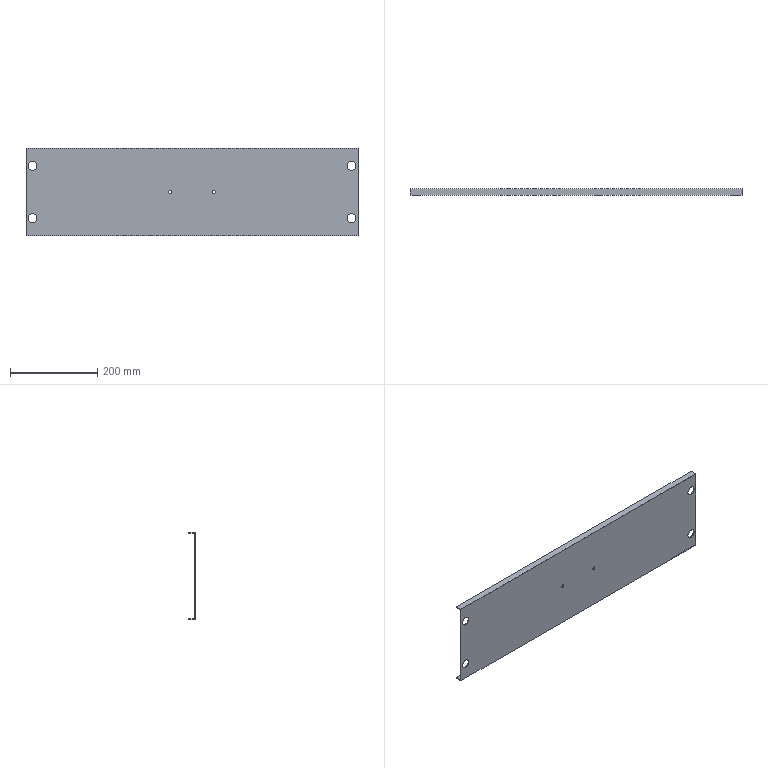Part | SolidWorks | features BaseBody 1 | 1 solid | 22 faces | box 760 x 15 x 200 mm | volume 340844 mm3 | cylinder 12 | plane 10 | commonest cylinder face diameters 20 x8 7.2 x4
STEP:
#1=CARTESIAN_POINT('',(181.946,-3036.473,1814.721));
#2=VERTEX_POINT('',#1);
#3=CARTESIAN_POINT('',(181.946,-3036.473,1794.721));
#4=VERTEX_POINT('',#3);
#5=CARTESIAN_POINT('',(181.946,-3036.473,1804.721));
#6=DIRECTION('',(0.,-1.,0.));
#7=DIRECTION('',(0.,0.,-1.));
#8=AXIS2_PLACEMENT_3D('',#5,#6,#7);
#9=CIRCLE('',#8,10.);
#10=EDGE_CURVE('',#2,#4,#9,.T.);
#11=ORIENTED_EDGE('',*,*,#10,.F.);
#12=CARTESIAN_POINT('',(181.946,-3038.473,1814.721));
#13=VERTEX_POINT('',#12);
#14=CARTESIAN_POINT('',(181.946,-3062.967,1814.721));
#15=DIRECTION('',(0.,-1.,0.));
#16=VECTOR('',#15,1000.);
#17=LINE('',#14,#16);
#18=EDGE_CURVE('',#2,#13,#17,.T.);
#19=ORIENTED_EDGE('',*,*,#18,.T.);
#20=CARTESIAN_POINT('',(181.946,-3038.473,1794.721));
#21=VERTEX_POINT('',#20);
#22=CARTESIAN_POINT('',(181.946,-3038.473,1804.721));
#23=DIRECTION('',(0.,1.,0.));
#24=DIRECTION('',(0.,0.,-1.));
#25=AXIS2_PLACEMENT_3D('',#22,#23,#24);
#26=CIRCLE('',#25,10.);
#27=EDGE_CURVE('',#21,#13,#26,.T.);
#28=ORIENTED_EDGE('',*,*,#27,.F.);
#29=CARTESIAN_POINT('',(181.946,-3062.967,1794.721));
#30=DIRECTION('',(0.,-1.,0.));
#31=VECTOR('',#30,1000.);
#32=LINE('',#29,#31);
#33=EDGE_CURVE('',#4,#21,#32,.T.);
#34=ORIENTED_EDGE('',*,*,#33,.F.);
#35=EDGE_LOOP('',(#11,#19,#28,#34));
#36=FACE_OUTER_BOUND('',#35,.T.);
#37=CARTESIAN_POINT('',(181.946,-3062.967,1804.721));
#38=DIRECTION('',(0.,-1.,0.));
#39=DIRECTION('',(0.,0.,-1.));
#40=AXIS2_PLACEMENT_3D('',#37,#38,#39);
#41=CYLINDRICAL_SURFACE('',#40,10.);
#42=ADVANCED_FACE('',(#36),#41,.F.);
#43=CARTESIAN_POINT('',(911.946,-3038.473,1794.721));
#44=VERTEX_POINT('',#43);
#45=CARTESIAN_POINT('',(911.946,-3038.473,1814.721));
#46=VERTEX_POINT('',#45);
#47=CARTESIAN_POINT('',(911.946,-3038.473,1804.721));
#48=DIRECTION('',(0.,1.,0.));
#49=DIRECTION('',(0.,0.,1.));
#50=AXIS2_PLACEMENT_3D('',#47,#48,#49);
#51=CIRCLE('',#50,10.);
#52=EDGE_CURVE('',#44,#46,#51,.T.);
#53=ORIENTED_EDGE('',*,*,#52,.F.);
#54=CARTESIAN_POINT('',(911.946,-3036.473,1794.721));
#55=VERTEX_POINT('',#54);
#56=CARTESIAN_POINT('',(911.946,-3062.967,1794.721));
#57=DIRECTION('',(0.,1.,0.));
#58=VECTOR('',#57,1000.);
#59=LINE('',#56,#58);
#60=EDGE_CURVE('',#44,#55,#59,.T.);
#61=ORIENTED_EDGE('',*,*,#60,.T.);
#62=CARTESIAN_POINT('',(911.946,-3036.473,1814.721));
#63=VERTEX_POINT('',#62);
#64=CARTESIAN_POINT('',(911.946,-3036.473,1804.721));
#65=DIRECTION('',(0.,-1.,0.));
#66=DIRECTION('',(0.,0.,1.));
#67=AXIS2_PLACEMENT_3D('',#64,#65,#66);
#68=CIRCLE('',#67,10.);
#69=EDGE_CURVE('',#63,#55,#68,.T.);
#70=ORIENTED_EDGE('',*,*,#69,.F.);
#71=CARTESIAN_POINT('',(911.946,-3062.967,1814.721));
#72=DIRECTION('',(0.,1.,0.));
#73=VECTOR('',#72,1000.);
#74=LINE('',#71,#73);
#75=EDGE_CURVE('',#46,#63,#74,.T.);
#76=ORIENTED_EDGE('',*,*,#75,.F.);
#77=EDGE_LOOP('',(#53,#61,#70,#76));
#78=FACE_OUTER_BOUND('',#77,.T.);
#79=CARTESIAN_POINT('',(911.946,-3062.967,1804.721));
#80=DIRECTION('',(0.,1.,0.));
#81=DIRECTION('',(0.,0.,1.));
#82=AXIS2_PLACEMENT_3D('',#79,#80,#81);
#83=CYLINDRICAL_SURFACE('',#82,10.);
#84=ADVANCED_FACE('',(#78),#83,.F.);
#85=CARTESIAN_POINT('',(911.946,-3038.473,1674.721));
#86=VERTEX_POINT('',#85);
#87=CARTESIAN_POINT('',(911.946,-3038.473,1694.721));
#88=VERTEX_POINT('',#87);
#89=CARTESIAN_POINT('',(911.946,-3038.473,1684.721));
#90=DIRECTION('',(0.,1.,0.));
#91=DIRECTION('',(0.,0.,1.));
#92=AXIS2_PLACEMENT_3D('',#89,#90,#91);
#93=CIRCLE('',#92,10.);
#94=EDGE_CURVE('',#86,#88,#93,.T.);
#95=ORIENTED_EDGE('',*,*,#94,.F.);
#96=CARTESIAN_POINT('',(911.946,-3036.473,1674.721));
#97=VERTEX_POINT('',#96);
#98=CARTESIAN_POINT('',(911.946,-3062.967,1674.721));
#99=DIRECTION('',(0.,1.,0.));
#100=VECTOR('',#99,1000.);
#101=LINE('',#98,#100);
#102=EDGE_CURVE('',#86,#97,#101,.T.);
#103=ORIENTED_EDGE('',*,*,#102,.T.);
#104=CARTESIAN_POINT('',(911.946,-3036.473,1694.721));
#105=VERTEX_POINT('',#104);
#106=CARTESIAN_POINT('',(911.946,-3036.473,1684.721));
#107=DIRECTION('',(0.,-1.,0.));
#108=DIRECTION('',(0.,0.,1.));
#109=AXIS2_PLACEMENT_3D('',#106,#107,#108);
#110=CIRCLE('',#109,10.);
#111=EDGE_CURVE('',#105,#97,#110,.T.);
#112=ORIENTED_EDGE('',*,*,#111,.F.);
#113=CARTESIAN_POINT('',(911.946,-3062.967,1694.721));
#114=DIRECTION('',(0.,1.,0.));
#115=VECTOR('',#114,1000.);
#116=LINE('',#113,#115);
#117=EDGE_CURVE('',#88,#105,#116,.T.);
#118=ORIENTED_EDGE('',*,*,#117,.F.);
#119=EDGE_LOOP('',(#95,#103,#112,#118));
#120=FACE_OUTER_BOUND('',#119,.T.);
#121=CARTESIAN_POINT('',(911.946,-3062.967,1684.721));
#122=DIRECTION('',(0.,1.,0.));
#123=DIRECTION('',(0.,0.,1.));
#124=AXIS2_PLACEMENT_3D('',#121,#122,#123);
#125=CYLINDRICAL_SURFACE('',#124,10.);
#126=ADVANCED_FACE('',(#120),#125,.F.);
#127=CARTESIAN_POINT('',(181.946,-3036.473,1694.721));
#128=VERTEX_POINT('',#127);
#129=CARTESIAN_POINT('',(181.946,-3036.473,1674.721));
#130=VERTEX_POINT('',#129);
#131=CARTESIAN_POINT('',(181.946,-3036.473,1684.721));
#132=DIRECTION('',(0.,-1.,0.));
#133=DIRECTION('',(0.,0.,-1.));
#134=AXIS2_PLACEMENT_3D('',#131,#132,#133);
#135=CIRCLE('',#134,10.);
#136=EDGE_CURVE('',#128,#130,#135,.T.);
#137=ORIENTED_EDGE('',*,*,#136,.F.);
#138=CARTESIAN_POINT('',(181.946,-3038.473,1694.721));
#139=VERTEX_POINT('',#138);
#140=CARTESIAN_POINT('',(181.946,-3062.967,1694.721));
#141=DIRECTION('',(0.,-1.,0.));
#142=VECTOR('',#141,1000.);
#143=LINE('',#140,#142);
#144=EDGE_CURVE('',#128,#139,#143,.T.);
#145=ORIENTED_EDGE('',*,*,#144,.T.);
#146=CARTESIAN_POINT('',(181.946,-3038.473,1674.721));
#147=VERTEX_POINT('',#146);
#148=CARTESIAN_POINT('',(181.946,-3038.473,1684.721));
#149=DIRECTION('',(0.,1.,0.));
#150=DIRECTION('',(0.,0.,-1.));
#151=AXIS2_PLACEMENT_3D('',#148,#149,#150);
#152=CIRCLE('',#151,10.);
#153=EDGE_CURVE('',#147,#139,#152,.T.);
#154=ORIENTED_EDGE('',*,*,#153,.F.);
#155=CARTESIAN_POINT('',(181.946,-3062.967,1674.721));
#156=DIRECTION('',(0.,-1.,0.));
#157=VECTOR('',#156,1000.);
#158=LINE('',#155,#157);
#159=EDGE_CURVE('',#130,#147,#158,.T.);
#160=ORIENTED_EDGE('',*,*,#159,.F.);
#161=EDGE_LOOP('',(#137,#145,#154,#160));
#162=FACE_OUTER_BOUND('',#161,.T.);
#163=CARTESIAN_POINT('',(181.946,-3062.967,1684.721));
#164=DIRECTION('',(0.,-1.,0.));
#165=DIRECTION('',(0.,0.,-1.));
#166=AXIS2_PLACEMENT_3D('',#163,#164,#165);
#167=CYLINDRICAL_SURFACE('',#166,10.);
#168=ADVANCED_FACE('',(#162),#167,.F.);
#169=CARTESIAN_POINT('',(496.946,-3036.473,1748.321));
#170=VERTEX_POINT('',#169);
#171=CARTESIAN_POINT('',(496.946,-3036.473,1741.121));
#172=VERTEX_POINT('',#171);
#173=CARTESIAN_POINT('',(496.946,-3036.473,1744.721));
#174=DIRECTION('',(0.,-1.,0.));
#175=DIRECTION('',(0.,0.,-1.));
#176=AXIS2_PLACEMENT_3D('',#173,#174,#175);
#177=CIRCLE('',#176,3.6);
#178=EDGE_CURVE('',#170,#172,#177,.T.);
#179=ORIENTED_EDGE('',*,*,#178,.F.);
#180=CARTESIAN_POINT('',(496.946,-3038.473,1748.321));
#181=VERTEX_POINT('',#180);
#182=CARTESIAN_POINT('',(496.946,-3062.023,1748.321));
#183=DIRECTION('',(0.,-1.,0.));
#184=VECTOR('',#183,1000.);
#185=LINE('',#182,#184);
#186=EDGE_CURVE('',#170,#181,#185,.T.);
#187=ORIENTED_EDGE('',*,*,#186,.T.);
#188=CARTESIAN_POINT('',(496.946,-3038.473,1741.121));
#189=VERTEX_POINT('',#188);
#190=CARTESIAN_POINT('',(496.946,-3038.473,1744.721));
#191=DIRECTION('',(0.,1.,0.));
#192=DIRECTION('',(0.,0.,-1.));
#193=AXIS2_PLACEMENT_3D('',#190,#191,#192);
#194=CIRCLE('',#193,3.6);
#195=EDGE_CURVE('',#189,#181,#194,.T.);
#196=ORIENTED_EDGE('',*,*,#195,.F.);
#197=CARTESIAN_POINT('',(496.946,-3062.023,1741.121));
#198=DIRECTION('',(0.,-1.,0.));
#199=VECTOR('',#198,1000.);
#200=LINE('',#197,#199);
#201=EDGE_CURVE('',#172,#189,#200,.T.);
#202=ORIENTED_EDGE('',*,*,#201,.F.);
#203=EDGE_LOOP('',(#179,#187,#196,#202));
#204=FACE_OUTER_BOUND('',#203,.T.);
#205=CARTESIAN_POINT('',(496.946,-3062.023,1744.721));
#206=DIRECTION('',(0.,-1.,0.));
#207=DIRECTION('',(0.,0.,-1.));
#208=AXIS2_PLACEMENT_3D('',#205,#206,#207);
#209=CYLINDRICAL_SURFACE('',#208,3.6);
#210=ADVANCED_FACE('',(#204),#209,.F.);
#211=CARTESIAN_POINT('',(596.946,-3036.473,1748.321));
#212=VERTEX_POINT('',#211);
#213=CARTESIAN_POINT('',(596.946,-3036.473,1741.121));
#214=VERTEX_POINT('',#213);
#215=CARTESIAN_POINT('',(596.946,-3036.473,1744.721));
#216=DIRECTION('',(0.,-1.,0.));
#217=DIRECTION('',(0.,0.,-1.));
#218=AXIS2_PLACEMENT_3D('',#215,#216,#217);
#219=CIRCLE('',#218,3.6);
#220=EDGE_CURVE('',#212,#214,#219,.T.);
#221=ORIENTED_EDGE('',*,*,#220,.F.);
#222=CARTESIAN_POINT('',(596.946,-3038.473,1748.321));
#223=VERTEX_POINT('',#222);
#224=CARTESIAN_POINT('',(596.946,-3058.12,1748.321));
#225=DIRECTION('',(0.,-1.,0.));
#226=VECTOR('',#225,1000.);
#227=LINE('',#224,#226);
#228=EDGE_CURVE('',#212,#223,#227,.T.);
#229=ORIENTED_EDGE('',*,*,#228,.T.);
#230=CARTESIAN_POINT('',(596.946,-3038.473,1741.121));
#231=VERTEX_POINT('',#230);
#232=CARTESIAN_POINT('',(596.946,-3038.473,1744.721));
#233=DIRECTION('',(0.,1.,0.));
#234=DIRECTION('',(0.,0.,-1.));
#235=AXIS2_PLACEMENT_3D('',#232,#233,#234);
#236=CIRCLE('',#235,3.6);
#237=EDGE_CURVE('',#231,#223,#236,.T.);
#238=ORIENTED_EDGE('',*,*,#237,.F.);
#239=CARTESIAN_POINT('',(596.946,-3058.12,1741.121));
#240=DIRECTION('',(0.,-1.,0.));
#241=VECTOR('',#240,1000.);
#242=LINE('',#239,#241);
#243=EDGE_CURVE('',#214,#231,#242,.T.);
#244=ORIENTED_EDGE('',*,*,#243,.F.);
#245=EDGE_LOOP('',(#221,#229,#238,#244));
#246=FACE_OUTER_BOUND('',#245,.T.);
#247=CARTESIAN_POINT('',(596.946,-3058.12,1744.721));
#248=DIRECTION('',(0.,-1.,0.));
#249=DIRECTION('',(0.,0.,-1.));
#250=AXIS2_PLACEMENT_3D('',#247,#248,#249);
#251=CYLINDRICAL_SURFACE('',#250,3.6);
#252=ADVANCED_FACE('',(#246),#251,.F.);
#253=CARTESIAN_POINT('',(926.946,-3038.473,1644.721));
#254=VERTEX_POINT('',#253);
#255=CARTESIAN_POINT('',(926.946,-3038.473,1844.721));
#256=VERTEX_POINT('',#255);
#257=CARTESIAN_POINT('',(926.946,-3038.473,1844.721));
#258=DIRECTION('',(0.,0.,1.));
#259=VECTOR('',#258,1000.);
#260=LINE('',#257,#259);
#261=EDGE_CURVE('',#254,#256,#260,.T.);
#262=ORIENTED_EDGE('',*,*,#261,.T.);
#263=CARTESIAN_POINT('',(166.946,-3038.473,1844.721));
#264=VERTEX_POINT('',#263);
#265=CARTESIAN_POINT('',(926.946,-3038.473,1844.721));
#266=DIRECTION('',(-1.,0.,0.));
#267=VECTOR('',#266,1000.);
#268=LINE('',#265,#267);
#269=EDGE_CURVE('',#256,#264,#268,.T.);
#270=ORIENTED_EDGE('',*,*,#269,.T.);
#271=CARTESIAN_POINT('',(166.946,-3038.473,1644.721));
#272=VERTEX_POINT('',#271);
#273=CARTESIAN_POINT('',(166.946,-3038.473,1844.721));
#274=DIRECTION('',(0.,0.,-1.));
#275=VECTOR('',#274,1000.);
#276=LINE('',#273,#275);
#277=EDGE_CURVE('',#264,#272,#276,.T.);
#278=ORIENTED_EDGE('',*,*,#277,.T.);
#279=CARTESIAN_POINT('',(926.946,-3038.473,1644.721));
#280=DIRECTION('',(1.,0.,0.));
#281=VECTOR('',#280,1000.);
#282=LINE('',#279,#281);
#283=EDGE_CURVE('',#272,#254,#282,.T.);
#284=ORIENTED_EDGE('',*,*,#283,.T.);
#285=EDGE_LOOP('',(#262,#270,#278,#284));
#286=FACE_OUTER_BOUND('',#285,.T.);
#287=ORIENTED_EDGE('',*,*,#27,.T.);
#288=CARTESIAN_POINT('',(181.946,-3038.473,1804.721));
#289=DIRECTION('',(0.,1.,0.));
#290=DIRECTION('',(0.,0.,-1.));
#291=AXIS2_PLACEMENT_3D('',#288,#289,#290);
#292=CIRCLE('',#291,10.);
#293=EDGE_CURVE('',#13,#21,#292,.T.);
#294=ORIENTED_EDGE('',*,*,#293,.T.);
#295=EDGE_LOOP('',(#287,#294));
#296=FACE_BOUND('',#295,.T.);
#297=CARTESIAN_POINT('',(911.946,-3038.473,1804.721));
#298=DIRECTION('',(0.,1.,0.));
#299=DIRECTION('',(0.,0.,1.));
#300=AXIS2_PLACEMENT_3D('',#297,#298,#299);
#301=CIRCLE('',#300,10.);
#302=EDGE_CURVE('',#46,#44,#301,.T.);
#303=ORIENTED_EDGE('',*,*,#302,.T.);
#304=ORIENTED_EDGE('',*,*,#52,.T.);
#305=EDGE_LOOP('',(#303,#304));
#306=FACE_BOUND('',#305,.T.);
#307=CARTESIAN_POINT('',(911.946,-3038.473,1684.721));
#308=DIRECTION('',(0.,1.,0.));
#309=DIRECTION('',(0.,0.,1.));
#310=AXIS2_PLACEMENT_3D('',#307,#308,#309);
#311=CIRCLE('',#310,10.);
#312=EDGE_CURVE('',#88,#86,#311,.T.);
#313=ORIENTED_EDGE('',*,*,#312,.T.);
#314=ORIENTED_EDGE('',*,*,#94,.T.);
#315=EDGE_LOOP('',(#313,#314));
#316=FACE_BOUND('',#315,.T.);
#317=ORIENTED_EDGE('',*,*,#153,.T.);
#318=CARTESIAN_POINT('',(181.946,-3038.473,1684.721));
#319=DIRECTION('',(0.,1.,0.));
#320=DIRECTION('',(0.,0.,-1.));
#321=AXIS2_PLACEMENT_3D('',#318,#319,#320);
#322=CIRCLE('',#321,10.);
#323=EDGE_CURVE('',#139,#147,#322,.T.);
#324=ORIENTED_EDGE('',*,*,#323,.T.);
#325=EDGE_LOOP('',(#317,#324));
#326=FACE_BOUND('',#325,.T.);
#327=ORIENTED_EDGE('',*,*,#195,.T.);
#328=CARTESIAN_POINT('',(496.946,-3038.473,1744.721));
#329=DIRECTION('',(0.,1.,0.));
#330=DIRECTION('',(0.,0.,-1.));
#331=AXIS2_PLACEMENT_3D('',#328,#329,#330);
#332=CIRCLE('',#331,3.6);
#333=EDGE_CURVE('',#181,#189,#332,.T.);
#334=ORIENTED_EDGE('',*,*,#333,.T.);
#335=EDGE_LOOP('',(#327,#334));
#336=FACE_BOUND('',#335,.T.);
#337=ORIENTED_EDGE('',*,*,#237,.T.);
#338=CARTESIAN_POINT('',(596.946,-3038.473,1744.721));
#339=DIRECTION('',(0.,1.,0.));
#340=DIRECTION('',(0.,0.,-1.));
#341=AXIS2_PLACEMENT_3D('',#338,#339,#340);
#342=CIRCLE('',#341,3.6);
#343=EDGE_CURVE('',#223,#231,#342,.T.);
#344=ORIENTED_EDGE('',*,*,#343,.T.);
#345=EDGE_LOOP('',(#337,#344));
#346=FACE_BOUND('',#345,.T.);
#347=CARTESIAN_POINT('',(926.946,-3038.473,1844.721));
#348=DIRECTION('',(0.,-1.,0.));
#349=DIRECTION('',(0.,0.,-1.));
#350=AXIS2_PLACEMENT_3D('',#347,#348,#349);
#351=PLANE('',#350);
#352=ADVANCED_FACE('',(#286,#296,#306,#316,#326,#336,#346),#351,.T.);
#353=CARTESIAN_POINT('',(926.946,-3023.473,1844.721));
#354=VERTEX_POINT('',#353);
#355=CARTESIAN_POINT('',(926.946,-3023.473,1844.721));
#356=DIRECTION('',(0.,1.,0.));
#357=VECTOR('',#356,1000.);
#358=LINE('',#355,#357);
#359=EDGE_CURVE('',#256,#354,#358,.T.);
#360=ORIENTED_EDGE('',*,*,#359,.T.);
#361=CARTESIAN_POINT('',(166.946,-3023.473,1844.721));
#362=VERTEX_POINT('',#361);
#363=CARTESIAN_POINT('',(926.946,-3023.473,1844.721));
#364=DIRECTION('',(-1.,0.,0.));
#365=VECTOR('',#364,1000.);
#366=LINE('',#363,#365);
#367=EDGE_CURVE('',#354,#362,#366,.T.);
#368=ORIENTED_EDGE('',*,*,#367,.T.);
#369=CARTESIAN_POINT('',(166.946,-3023.473,1844.721));
#370=DIRECTION('',(0.,-1.,0.));
#371=VECTOR('',#370,1000.);
#372=LINE('',#369,#371);
#373=EDGE_CURVE('',#362,#264,#372,.T.);
#374=ORIENTED_EDGE('',*,*,#373,.T.);
#375=ORIENTED_EDGE('',*,*,#269,.F.);
#376=EDGE_LOOP('',(#360,#368,#374,#375));
#377=FACE_OUTER_BOUND('',#376,.T.);
#378=CARTESIAN_POINT('',(926.946,-3023.473,1844.721));
#379=DIRECTION('',(0.,0.,1.));
#380=DIRECTION('',(1.,0.,0.));
#381=AXIS2_PLACEMENT_3D('',#378,#379,#380);
#382=PLANE('',#381);
#383=ADVANCED_FACE('',(#377),#382,.T.);
#384=ORIENTED_EDGE('',*,*,#359,.F.);
#385=ORIENTED_EDGE('',*,*,#261,.F.);
#386=CARTESIAN_POINT('',(926.946,-3023.473,1644.721));
#387=VERTEX_POINT('',#386);
#388=CARTESIAN_POINT('',(926.946,-3036.504,1644.721));
#389=DIRECTION('',(0.,1.,0.));
#390=VECTOR('',#389,1000.);
#391=LINE('',#388,#390);
#392=EDGE_CURVE('',#254,#387,#391,.T.);
#393=ORIENTED_EDGE('',*,*,#392,.T.);
#394=CARTESIAN_POINT('',(926.946,-3023.473,1646.721));
#395=VERTEX_POINT('',#394);
#396=CARTESIAN_POINT('',(926.946,-3023.473,1744.721));
#397=DIRECTION('',(0.,0.,1.));
#398=VECTOR('',#397,1000.);
#399=LINE('',#396,#398);
#400=EDGE_CURVE('',#387,#395,#399,.T.);
#401=ORIENTED_EDGE('',*,*,#400,.T.);
#402=CARTESIAN_POINT('',(926.946,-3036.473,1646.721));
#403=VERTEX_POINT('',#402);
#404=CARTESIAN_POINT('',(926.946,-3036.504,1646.721));
#405=DIRECTION('',(0.,-1.,0.));
#406=VECTOR('',#405,1000.);
#407=LINE('',#404,#406);
#408=EDGE_CURVE('',#395,#403,#407,.T.);
#409=ORIENTED_EDGE('',*,*,#408,.T.);
#410=CARTESIAN_POINT('',(926.946,-3036.473,1842.721));
#411=VERTEX_POINT('',#410);
#412=CARTESIAN_POINT('',(926.946,-3036.473,1744.721));
#413=DIRECTION('',(0.,0.,1.));
#414=VECTOR('',#413,1000.);
#415=LINE('',#412,#414);
#416=EDGE_CURVE('',#403,#411,#415,.T.);
#417=ORIENTED_EDGE('',*,*,#416,.T.);
#418=CARTESIAN_POINT('',(926.946,-3023.473,1842.721));
#419=VERTEX_POINT('',#418);
#420=CARTESIAN_POINT('',(926.946,-3036.504,1842.721));
#421=DIRECTION('',(0.,1.,0.));
#422=VECTOR('',#421,1000.);
#423=LINE('',#420,#422);
#424=EDGE_CURVE('',#411,#419,#423,.T.);
#425=ORIENTED_EDGE('',*,*,#424,.T.);
#426=CARTESIAN_POINT('',(926.946,-3023.473,1744.721));
#427=DIRECTION('',(0.,0.,1.));
#428=VECTOR('',#427,1000.);
#429=LINE('',#426,#428);
#430=EDGE_CURVE('',#419,#354,#429,.T.);
#431=ORIENTED_EDGE('',*,*,#430,.T.);
#432=EDGE_LOOP('',(#384,#385,#393,#401,#409,#417,#425,#431));
#433=FACE_OUTER_BOUND('',#432,.T.);
#434=CARTESIAN_POINT('',(926.946,-3036.504,1744.721));
#435=DIRECTION('',(1.,0.,0.));
#436=DIRECTION('',(0.,0.,-1.));
#437=AXIS2_PLACEMENT_3D('',#434,#435,#436);
#438=PLANE('',#437);
#439=ADVANCED_FACE('',(#433),#438,.T.);
#440=ORIENTED_EDGE('',*,*,#392,.F.);
#441=ORIENTED_EDGE('',*,*,#283,.F.);
#442=CARTESIAN_POINT('',(166.946,-3023.473,1644.721));
#443=VERTEX_POINT('',#442);
#444=CARTESIAN_POINT('',(166.946,-3038.473,1644.721));
#445=DIRECTION('',(0.,1.,0.));
#446=VECTOR('',#445,1000.);
#447=LINE('',#444,#446);
#448=EDGE_CURVE('',#272,#443,#447,.T.);
#449=ORIENTED_EDGE('',*,*,#448,.T.);
#450=CARTESIAN_POINT('',(926.946,-3023.473,1644.721));
#451=DIRECTION('',(1.,0.,0.));
#452=VECTOR('',#451,1000.);
#453=LINE('',#450,#452);
#454=EDGE_CURVE('',#443,#387,#453,.T.);
#455=ORIENTED_EDGE('',*,*,#454,.T.);
#456=EDGE_LOOP('',(#440,#441,#449,#455));
#457=FACE_OUTER_BOUND('',#456,.T.);
#458=CARTESIAN_POINT('',(926.946,-3038.473,1644.721));
#459=DIRECTION('',(0.,0.,-1.));
#460=DIRECTION('',(-1.,0.,0.));
#461=AXIS2_PLACEMENT_3D('',#458,#459,#460);
#462=PLANE('',#461);
#463=ADVANCED_FACE('',(#457),#462,.T.);
#464=ORIENTED_EDGE('',*,*,#448,.F.);
#465=ORIENTED_EDGE('',*,*,#277,.F.);
#466=ORIENTED_EDGE('',*,*,#373,.F.);
#467=CARTESIAN_POINT('',(166.946,-3023.473,1842.721));
#468=VERTEX_POINT('',#467);
#469=CARTESIAN_POINT('',(166.946,-3023.473,1744.721));
#470=DIRECTION('',(0.,0.,1.));
#471=VECTOR('',#470,1000.);
#472=LINE('',#469,#471);
#473=EDGE_CURVE('',#468,#362,#472,.T.);
#474=ORIENTED_EDGE('',*,*,#473,.F.);
#475=CARTESIAN_POINT('',(166.946,-3036.473,1842.721));
#476=VERTEX_POINT('',#475);
#477=CARTESIAN_POINT('',(166.946,-3036.504,1842.721));
#478=DIRECTION('',(0.,1.,0.));
#479=VECTOR('',#478,1000.);
#480=LINE('',#477,#479);
#481=EDGE_CURVE('',#476,#468,#480,.T.);
#482=ORIENTED_EDGE('',*,*,#481,.F.);
#483=CARTESIAN_POINT('',(166.946,-3036.473,1646.721));
#484=VERTEX_POINT('',#483);
#485=CARTESIAN_POINT('',(166.946,-3036.473,1744.721));
#486=DIRECTION('',(0.,0.,1.));
#487=VECTOR('',#486,1000.);
#488=LINE('',#485,#487);
#489=EDGE_CURVE('',#484,#476,#488,.T.);
#490=ORIENTED_EDGE('',*,*,#489,.F.);
#491=CARTESIAN_POINT('',(166.946,-3023.473,1646.721));
#492=VERTEX_POINT('',#491);
#493=CARTESIAN_POINT('',(166.946,-3036.504,1646.721));
#494=DIRECTION('',(0.,-1.,0.));
#495=VECTOR('',#494,1000.);
#496=LINE('',#493,#495);
#497=EDGE_CURVE('',#492,#484,#496,.T.);
#498=ORIENTED_EDGE('',*,*,#497,.F.);
#499=CARTESIAN_POINT('',(166.946,-3023.473,1744.721));
#500=DIRECTION('',(0.,0.,1.));
#501=VECTOR('',#500,1000.);
#502=LINE('',#499,#501);
#503=EDGE_CURVE('',#443,#492,#502,.T.);
#504=ORIENTED_EDGE('',*,*,#503,.F.);
#505=EDGE_LOOP('',(#464,#465,#466,#474,#482,#490,#498,#504));
#506=FACE_OUTER_BOUND('',#505,.T.);
#507=CARTESIAN_POINT('',(166.946,-3036.504,1744.721));
#508=DIRECTION('',(1.,0.,0.));
#509=DIRECTION('',(0.,0.,-1.));
#510=AXIS2_PLACEMENT_3D('',#507,#508,#509);
#511=PLANE('',#510);
#512=ADVANCED_FACE('',(#506),#511,.F.);
#513=ORIENTED_EDGE('',*,*,#18,.F.);
#514=CARTESIAN_POINT('',(181.946,-3036.473,1804.721));
#515=DIRECTION('',(0.,-1.,0.));
#516=DIRECTION('',(0.,0.,-1.));
#517=AXIS2_PLACEMENT_3D('',#514,#515,#516);
#518=CIRCLE('',#517,10.);
#519=EDGE_CURVE('',#4,#2,#518,.T.);
#520=ORIENTED_EDGE('',*,*,#519,.F.);
#521=ORIENTED_EDGE('',*,*,#33,.T.);
#522=ORIENTED_EDGE('',*,*,#293,.F.);
#523=EDGE_LOOP('',(#513,#520,#521,#522));
#524=FACE_OUTER_BOUND('',#523,.T.);
#525=CARTESIAN_POINT('',(181.946,-3062.967,1804.721));
#526=DIRECTION('',(0.,-1.,0.));
#527=DIRECTION('',(0.,0.,-1.));
#528=AXIS2_PLACEMENT_3D('',#525,#526,#527);
#529=CYLINDRICAL_SURFACE('',#528,10.);
#530=ADVANCED_FACE('',(#524),#529,.F.);
#531=ORIENTED_EDGE('',*,*,#60,.F.);
#532=ORIENTED_EDGE('',*,*,#302,.F.);
#533=ORIENTED_EDGE('',*,*,#75,.T.);
#534=CARTESIAN_POINT('',(911.946,-3036.473,1804.721));
#535=DIRECTION('',(0.,-1.,0.));
#536=DIRECTION('',(0.,0.,1.));
#537=AXIS2_PLACEMENT_3D('',#534,#535,#536);
#538=CIRCLE('',#537,10.);
#539=EDGE_CURVE('',#55,#63,#538,.T.);
#540=ORIENTED_EDGE('',*,*,#539,.F.);
#541=EDGE_LOOP('',(#531,#532,#533,#540));
#542=FACE_OUTER_BOUND('',#541,.T.);
#543=CARTESIAN_POINT('',(911.946,-3062.967,1804.721));
#544=DIRECTION('',(0.,1.,0.));
#545=DIRECTION('',(0.,0.,1.));
#546=AXIS2_PLACEMENT_3D('',#543,#544,#545);
#547=CYLINDRICAL_SURFACE('',#546,10.);
#548=ADVANCED_FACE('',(#542),#547,.F.);
#549=ORIENTED_EDGE('',*,*,#102,.F.);
#550=ORIENTED_EDGE('',*,*,#312,.F.);
#551=ORIENTED_EDGE('',*,*,#117,.T.);
#552=CARTESIAN_POINT('',(911.946,-3036.473,1684.721));
#553=DIRECTION('',(0.,-1.,0.));
#554=DIRECTION('',(0.,0.,1.));
#555=AXIS2_PLACEMENT_3D('',#552,#553,#554);
#556=CIRCLE('',#555,10.);
#557=EDGE_CURVE('',#97,#105,#556,.T.);
#558=ORIENTED_EDGE('',*,*,#557,.F.);
#559=EDGE_LOOP('',(#549,#550,#551,#558));
#560=FACE_OUTER_BOUND('',#559,.T.);
#561=CARTESIAN_POINT('',(911.946,-3062.967,1684.721));
#562=DIRECTION('',(0.,1.,0.));
#563=DIRECTION('',(0.,0.,1.));
#564=AXIS2_PLACEMENT_3D('',#561,#562,#563);
#565=CYLINDRICAL_SURFACE('',#564,10.);
#566=ADVANCED_FACE('',(#560),#565,.F.);
#567=ORIENTED_EDGE('',*,*,#144,.F.);
#568=CARTESIAN_POINT('',(181.946,-3036.473,1684.721));
#569=DIRECTION('',(0.,-1.,0.));
#570=DIRECTION('',(0.,0.,-1.));
#571=AXIS2_PLACEMENT_3D('',#568,#569,#570);
#572=CIRCLE('',#571,10.);
#573=EDGE_CURVE('',#130,#128,#572,.T.);
#574=ORIENTED_EDGE('',*,*,#573,.F.);
#575=ORIENTED_EDGE('',*,*,#159,.T.);
#576=ORIENTED_EDGE('',*,*,#323,.F.);
#577=EDGE_LOOP('',(#567,#574,#575,#576));
#578=FACE_OUTER_BOUND('',#577,.T.);
#579=CARTESIAN_POINT('',(181.946,-3062.967,1684.721));
#580=DIRECTION('',(0.,-1.,0.));
#581=DIRECTION('',(0.,0.,-1.));
#582=AXIS2_PLACEMENT_3D('',#579,#580,#581);
#583=CYLINDRICAL_SURFACE('',#582,10.);
#584=ADVANCED_FACE('',(#578),#583,.F.);
#585=ORIENTED_EDGE('',*,*,#186,.F.);
#586=CARTESIAN_POINT('',(496.946,-3036.473,1744.721));
#587=DIRECTION('',(0.,-1.,0.));
#588=DIRECTION('',(0.,0.,-1.));
#589=AXIS2_PLACEMENT_3D('',#586,#587,#588);
#590=CIRCLE('',#589,3.6);
#591=EDGE_CURVE('',#172,#170,#590,.T.);
#592=ORIENTED_EDGE('',*,*,#591,.F.);
#593=ORIENTED_EDGE('',*,*,#201,.T.);
#594=ORIENTED_EDGE('',*,*,#333,.F.);
#595=EDGE_LOOP('',(#585,#592,#593,#594));
#596=FACE_OUTER_BOUND('',#595,.T.);
#597=CARTESIAN_POINT('',(496.946,-3062.023,1744.721));
#598=DIRECTION('',(0.,-1.,0.));
#599=DIRECTION('',(0.,0.,-1.));
#600=AXIS2_PLACEMENT_3D('',#597,#598,#599);
#601=CYLINDRICAL_SURFACE('',#600,3.6);
#602=ADVANCED_FACE('',(#596),#601,.F.);
#603=ORIENTED_EDGE('',*,*,#228,.F.);
#604=CARTESIAN_POINT('',(596.946,-3036.473,1744.721));
#605=DIRECTION('',(0.,-1.,0.));
#606=DIRECTION('',(0.,0.,-1.));
#607=AXIS2_PLACEMENT_3D('',#604,#605,#606);
#608=CIRCLE('',#607,3.6);
#609=EDGE_CURVE('',#214,#212,#608,.T.);
#610=ORIENTED_EDGE('',*,*,#609,.F.);
#611=ORIENTED_EDGE('',*,*,#243,.T.);
#612=ORIENTED_EDGE('',*,*,#343,.F.);
#613=EDGE_LOOP('',(#603,#610,#611,#612));
#614=FACE_OUTER_BOUND('',#613,.T.);
#615=CARTESIAN_POINT('',(596.946,-3058.12,1744.721));
#616=DIRECTION('',(0.,-1.,0.));
#617=DIRECTION('',(0.,0.,-1.));
#618=AXIS2_PLACEMENT_3D('',#615,#616,#617);
#619=CYLINDRICAL_SURFACE('',#618,3.6);
#620=ADVANCED_FACE('',(#614),#619,.F.);
#621=ORIENTED_EDGE('',*,*,#430,.F.);
#622=CARTESIAN_POINT('',(926.946,-3023.473,1842.721));
#623=DIRECTION('',(-1.,0.,0.));
#624=VECTOR('',#623,1000.);
#625=LINE('',#622,#624);
#626=EDGE_CURVE('',#419,#468,#625,.T.);
#627=ORIENTED_EDGE('',*,*,#626,.T.);
#628=ORIENTED_EDGE('',*,*,#473,.T.);
#629=ORIENTED_EDGE('',*,*,#367,.F.);
#630=EDGE_LOOP('',(#621,#627,#628,#629));
#631=FACE_OUTER_BOUND('',#630,.T.);
#632=CARTESIAN_POINT('',(926.946,-3023.473,1842.721));
#633=DIRECTION('',(0.,1.,0.));
#634=DIRECTION('',(0.,0.,1.));
#635=AXIS2_PLACEMENT_3D('',#632,#633,#634);
#636=PLANE('',#635);
#637=ADVANCED_FACE('',(#631),#636,.T.);
#638=ORIENTED_EDGE('',*,*,#424,.F.);
#639=CARTESIAN_POINT('',(926.946,-3036.473,1842.721));
#640=DIRECTION('',(-1.,0.,0.));
#641=VECTOR('',#640,1000.);
#642=LINE('',#639,#641);
#643=EDGE_CURVE('',#411,#476,#642,.T.);
#644=ORIENTED_EDGE('',*,*,#643,.T.);
#645=ORIENTED_EDGE('',*,*,#481,.T.);
#646=ORIENTED_EDGE('',*,*,#626,.F.);
#647=EDGE_LOOP('',(#638,#644,#645,#646));
#648=FACE_OUTER_BOUND('',#647,.T.);
#649=CARTESIAN_POINT('',(926.946,-3036.473,1842.721));
#650=DIRECTION('',(0.,0.,-1.));
#651=DIRECTION('',(-1.,0.,0.));
#652=AXIS2_PLACEMENT_3D('',#649,#650,#651);
#653=PLANE('',#652);
#654=ADVANCED_FACE('',(#648),#653,.T.);
#655=ORIENTED_EDGE('',*,*,#416,.F.);
#656=CARTESIAN_POINT('',(926.946,-3036.473,1646.721));
#657=DIRECTION('',(-1.,0.,0.));
#658=VECTOR('',#657,1000.);
#659=LINE('',#656,#658);
#660=EDGE_CURVE('',#403,#484,#659,.T.);
#661=ORIENTED_EDGE('',*,*,#660,.T.);
#662=ORIENTED_EDGE('',*,*,#489,.T.);
#663=ORIENTED_EDGE('',*,*,#643,.F.);
#664=EDGE_LOOP('',(#655,#661,#662,#663));
#665=FACE_OUTER_BOUND('',#664,.T.);
#666=ORIENTED_EDGE('',*,*,#519,.T.);
#667=ORIENTED_EDGE('',*,*,#10,.T.);
#668=EDGE_LOOP('',(#666,#667));
#669=FACE_BOUND('',#668,.T.);
#670=ORIENTED_EDGE('',*,*,#69,.T.);
#671=ORIENTED_EDGE('',*,*,#539,.T.);
#672=EDGE_LOOP('',(#670,#671));
#673=FACE_BOUND('',#672,.T.);
#674=ORIENTED_EDGE('',*,*,#111,.T.);
#675=ORIENTED_EDGE('',*,*,#557,.T.);
#676=EDGE_LOOP('',(#674,#675));
#677=FACE_BOUND('',#676,.T.);
#678=ORIENTED_EDGE('',*,*,#573,.T.);
#679=ORIENTED_EDGE('',*,*,#136,.T.);
#680=EDGE_LOOP('',(#678,#679));
#681=FACE_BOUND('',#680,.T.);
#682=ORIENTED_EDGE('',*,*,#591,.T.);
#683=ORIENTED_EDGE('',*,*,#178,.T.);
#684=EDGE_LOOP('',(#682,#683));
#685=FACE_BOUND('',#684,.T.);
#686=ORIENTED_EDGE('',*,*,#609,.T.);
#687=ORIENTED_EDGE('',*,*,#220,.T.);
#688=EDGE_LOOP('',(#686,#687));
#689=FACE_BOUND('',#688,.T.);
#690=CARTESIAN_POINT('',(926.946,-3036.473,1646.721));
#691=DIRECTION('',(0.,1.,0.));
#692=DIRECTION('',(0.,0.,1.));
#693=AXIS2_PLACEMENT_3D('',#690,#691,#692);
#694=PLANE('',#693);
#695=ADVANCED_FACE('',(#665,#669,#673,#677,#681,#685,#689),#694,.T.);
#696=ORIENTED_EDGE('',*,*,#408,.F.);
#697=CARTESIAN_POINT('',(926.946,-3023.473,1646.721));
#698=DIRECTION('',(-1.,0.,0.));
#699=VECTOR('',#698,1000.);
#700=LINE('',#697,#699);
#701=EDGE_CURVE('',#395,#492,#700,.T.);
#702=ORIENTED_EDGE('',*,*,#701,.T.);
#703=ORIENTED_EDGE('',*,*,#497,.T.);
#704=ORIENTED_EDGE('',*,*,#660,.F.);
#705=EDGE_LOOP('',(#696,#702,#703,#704));
#706=FACE_OUTER_BOUND('',#705,.T.);
#707=CARTESIAN_POINT('',(926.946,-3023.473,1646.721));
#708=DIRECTION('',(0.,0.,1.));
#709=DIRECTION('',(1.,0.,0.));
#710=AXIS2_PLACEMENT_3D('',#707,#708,#709);
#711=PLANE('',#710);
#712=ADVANCED_FACE('',(#706),#711,.T.);
#713=ORIENTED_EDGE('',*,*,#400,.F.);
#714=ORIENTED_EDGE('',*,*,#454,.F.);
#715=ORIENTED_EDGE('',*,*,#503,.T.);
#716=ORIENTED_EDGE('',*,*,#701,.F.);
#717=EDGE_LOOP('',(#713,#714,#715,#716));
#718=FACE_OUTER_BOUND('',#717,.T.);
#719=CARTESIAN_POINT('',(926.946,-3023.473,1644.721));
#720=DIRECTION('',(0.,1.,0.));
#721=DIRECTION('',(0.,0.,1.));
#722=AXIS2_PLACEMENT_3D('',#719,#720,#721);
#723=PLANE('',#722);
#724=ADVANCED_FACE('',(#718),#723,.T.);
#725=CLOSED_SHELL('',(#42,#84,#126,#168,#210,#252,#352,#383,#439,#463,#512,#530,#548,#566,#584,#602,#620,#637,#654,#695,#712,#724));
#726=MANIFOLD_SOLID_BREP('',#725);
#727=CARTESIAN_POINT('',(0.,0.,0.));
#728=DIRECTION('',(0.,0.,1.));
#729=DIRECTION('',(1.,0.,0.));
#730=AXIS2_PLACEMENT_3D('',#727,#728,#729);
#731=(LENGTH_UNIT()NAMED_UNIT(*)SI_UNIT(.MILLI.,.METRE.));
#732=UNCERTAINTY_MEASURE_WITH_UNIT(LENGTH_MEASURE(0.00001),#731,'','');
#733=(NAMED_UNIT(*)PLANE_ANGLE_UNIT()SI_UNIT($,.RADIAN.));
#734=(NAMED_UNIT(*)SI_UNIT($,.STERADIAN.)SOLID_ANGLE_UNIT());
#735=(GEOMETRIC_REPRESENTATION_CONTEXT(3)GLOBAL_UNCERTAINTY_ASSIGNED_CONTEXT((#732))GLOBAL_UNIT_ASSIGNED_CONTEXT((#731,#733,#734))REPRESENTATION_CONTEXT('',''));
#736=ADVANCED_BREP_SHAPE_REPRESENTATION('',(#726,#730),#735);